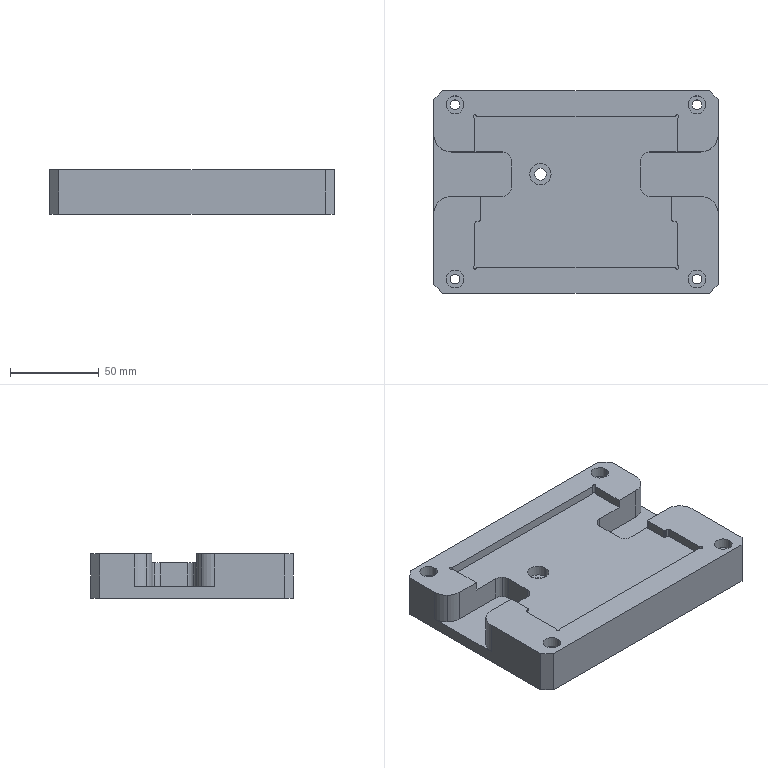Part | STEP file | ASND-0110-Body 1-10 | 1 solid | 89 faces | box 160 x 114 x 25 mm | volume 365953 mm3 | cylinder 54 | plane 35 | commonest cylinder face diameters 2 x18 10 x16 5.5 x8 20 x8 6.647 x2 12 x2